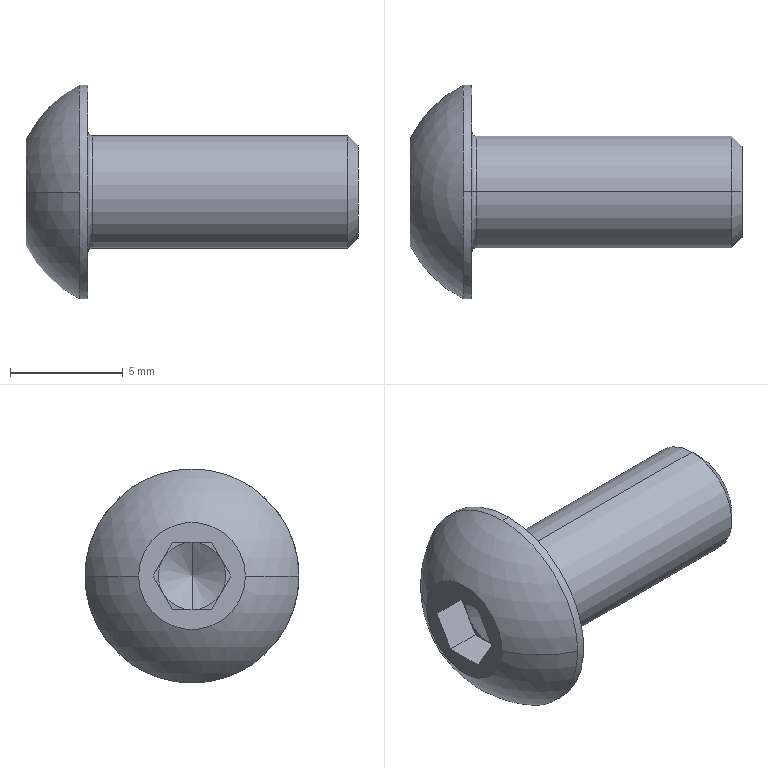Part | STEP file | SOCKET_BUTTON_HEAD_SCREW_ISO_IS | 1 solid | 27 faces | box 14.75 x 9.5 x 9.5 mm | volume 358.994 mm3 | plane 15 | cone 4 | cylinder 4 | torus 2 | sphere 2 | commonest cylinder face diameters 5 x2 9.5 x2
STEP:
#1=CARTESIAN_POINT('',(2.75,0.,2.7));
#2=VERTEX_POINT('',#1);
#3=CARTESIAN_POINT('',(2.75,0.,-2.7));
#4=VERTEX_POINT('',#3);
#5=CARTESIAN_POINT('',(2.75,0.,0.));
#6=DIRECTION('',(-1.,0.,0.));
#7=DIRECTION('',(0.,0.,1.));
#8=AXIS2_PLACEMENT_3D('',#5,#6,#7);
#9=CIRCLE('',#8,2.7);
#10=EDGE_CURVE('',#2,#4,#9,.T.);
#11=ORIENTED_EDGE('',*,*,#10,.F.);
#12=CARTESIAN_POINT('',(2.95,0.,2.5));
#13=VERTEX_POINT('',#12);
#14=CARTESIAN_POINT('',(2.95,0.,2.7));
#15=DIRECTION('',(0.,1.,0.));
#16=DIRECTION('',(0.,0.,-1.));
#17=AXIS2_PLACEMENT_3D('',#14,#15,#16);
#18=CIRCLE('',#17,0.2);
#19=EDGE_CURVE('',#13,#2,#18,.T.);
#20=ORIENTED_EDGE('',*,*,#19,.F.);
#21=CARTESIAN_POINT('',(2.95,0.,-2.5));
#22=VERTEX_POINT('',#21);
#23=CARTESIAN_POINT('',(2.95,0.,0.));
#24=DIRECTION('',(-1.,0.,0.));
#25=DIRECTION('',(0.,0.,1.));
#26=AXIS2_PLACEMENT_3D('',#23,#24,#25);
#27=CIRCLE('',#26,2.5);
#28=EDGE_CURVE('',#13,#22,#27,.T.);
#29=ORIENTED_EDGE('',*,*,#28,.T.);
#30=CARTESIAN_POINT('',(2.95,0.,-2.7));
#31=DIRECTION('',(0.,-1.,0.));
#32=DIRECTION('',(0.,0.,1.));
#33=AXIS2_PLACEMENT_3D('',#30,#31,#32);
#34=CIRCLE('',#33,0.2);
#35=EDGE_CURVE('',#22,#4,#34,.T.);
#36=ORIENTED_EDGE('',*,*,#35,.T.);
#37=EDGE_LOOP('',(#11,#20,#29,#36));
#38=FACE_OUTER_BOUND('',#37,.T.);
#39=CARTESIAN_POINT('',(2.95,0.,0.));
#40=DIRECTION('',(-1.,0.,0.));
#41=DIRECTION('',(0.,0.,1.));
#42=AXIS2_PLACEMENT_3D('',#39,#40,#41);
#43=TOROIDAL_SURFACE('',#42,2.7,0.2);
#44=ADVANCED_FACE('',(#38),#43,.F.);
#45=CARTESIAN_POINT('',(1.56,1.299,0.75));
#46=VERTEX_POINT('',#45);
#47=CARTESIAN_POINT('',(1.56,1.732,0.));
#48=VERTEX_POINT('',#47);
#49=CARTESIAN_POINT('',(1.56,1.299,0.75));
#50=DIRECTION('',(0.,0.5,-0.866));
#51=VECTOR('',#50,1000.);
#52=LINE('',#49,#51);
#53=EDGE_CURVE('',#46,#48,#52,.T.);
#54=ORIENTED_EDGE('',*,*,#53,.T.);
#55=CARTESIAN_POINT('',(1.56,1.299,-0.75));
#56=VERTEX_POINT('',#55);
#57=CARTESIAN_POINT('',(1.56,1.732,0.));
#58=DIRECTION('',(0.,-0.5,-0.866));
#59=VECTOR('',#58,1000.);
#60=LINE('',#57,#59);
#61=EDGE_CURVE('',#48,#56,#60,.T.);
#62=ORIENTED_EDGE('',*,*,#61,.T.);
#63=CARTESIAN_POINT('',(1.56,0.,0.));
#64=DIRECTION('',(1.,0.,0.));
#65=DIRECTION('',(0.,0.866,-0.5));
#66=AXIS2_PLACEMENT_3D('',#63,#64,#65);
#67=CIRCLE('',#66,1.5);
#68=EDGE_CURVE('',#56,#46,#67,.T.);
#69=ORIENTED_EDGE('',*,*,#68,.T.);
#70=EDGE_LOOP('',(#54,#62,#69));
#71=FACE_OUTER_BOUND('',#70,.T.);
#72=CARTESIAN_POINT('',(1.56,-1.732,0.));
#73=DIRECTION('',(1.,0.,0.));
#74=DIRECTION('',(0.,1.,0.));
#75=AXIS2_PLACEMENT_3D('',#72,#73,#74);
#76=PLANE('',#75);
#77=ADVANCED_FACE('',(#71),#76,.F.);
#78=CARTESIAN_POINT('',(1.56,0.866,1.5));
#79=VERTEX_POINT('',#78);
#80=CARTESIAN_POINT('',(1.56,0.866,1.5));
#81=DIRECTION('',(0.,0.5,-0.866));
#82=VECTOR('',#81,1000.);
#83=LINE('',#80,#82);
#84=EDGE_CURVE('',#79,#46,#83,.T.);
#85=ORIENTED_EDGE('',*,*,#84,.F.);
#86=CARTESIAN_POINT('',(0.,0.866,1.5));
#87=VERTEX_POINT('',#86);
#88=CARTESIAN_POINT('',(0.,0.866,1.5));
#89=DIRECTION('',(1.,0.,0.));
#90=VECTOR('',#89,1000.);
#91=LINE('',#88,#90);
#92=EDGE_CURVE('',#87,#79,#91,.T.);
#93=ORIENTED_EDGE('',*,*,#92,.F.);
#94=CARTESIAN_POINT('',(0.,1.732,0.));
#95=VERTEX_POINT('',#94);
#96=CARTESIAN_POINT('',(0.,1.732,0.));
#97=DIRECTION('',(0.,-0.5,0.866));
#98=VECTOR('',#97,1000.);
#99=LINE('',#96,#98);
#100=EDGE_CURVE('',#95,#87,#99,.T.);
#101=ORIENTED_EDGE('',*,*,#100,.F.);
#102=CARTESIAN_POINT('',(0.,1.732,0.));
#103=DIRECTION('',(1.,0.,0.));
#104=VECTOR('',#103,1000.);
#105=LINE('',#102,#104);
#106=EDGE_CURVE('',#95,#48,#105,.T.);
#107=ORIENTED_EDGE('',*,*,#106,.T.);
#108=ORIENTED_EDGE('',*,*,#53,.F.);
#109=EDGE_LOOP('',(#85,#93,#101,#107,#108));
#110=FACE_OUTER_BOUND('',#109,.T.);
#111=CARTESIAN_POINT('',(1.56,0.866,1.5));
#112=DIRECTION('',(0.,-0.866,-0.5));
#113=DIRECTION('',(0.,0.5,-0.866));
#114=AXIS2_PLACEMENT_3D('',#111,#112,#113);
#115=PLANE('',#114);
#116=ADVANCED_FACE('',(#110),#115,.T.);
#117=CARTESIAN_POINT('',(1.56,0.866,-1.5));
#118=VERTEX_POINT('',#117);
#119=CARTESIAN_POINT('',(1.56,1.299,-0.75));
#120=DIRECTION('',(0.,-0.5,-0.866));
#121=VECTOR('',#120,1000.);
#122=LINE('',#119,#121);
#123=EDGE_CURVE('',#56,#118,#122,.T.);
#124=ORIENTED_EDGE('',*,*,#123,.T.);
#125=CARTESIAN_POINT('',(1.56,0.,-1.5));
#126=VERTEX_POINT('',#125);
#127=CARTESIAN_POINT('',(1.56,0.866,-1.5));
#128=DIRECTION('',(0.,-1.,0.));
#129=VECTOR('',#128,1000.);
#130=LINE('',#127,#129);
#131=EDGE_CURVE('',#118,#126,#130,.T.);
#132=ORIENTED_EDGE('',*,*,#131,.T.);
#133=CARTESIAN_POINT('',(1.56,0.,0.));
#134=DIRECTION('',(1.,0.,0.));
#135=DIRECTION('',(0.,0.,-1.));
#136=AXIS2_PLACEMENT_3D('',#133,#134,#135);
#137=CIRCLE('',#136,1.5);
#138=EDGE_CURVE('',#126,#56,#137,.T.);
#139=ORIENTED_EDGE('',*,*,#138,.T.);
#140=EDGE_LOOP('',(#124,#132,#139));
#141=FACE_OUTER_BOUND('',#140,.T.);
#142=CARTESIAN_POINT('',(1.56,-1.732,0.));
#143=DIRECTION('',(1.,0.,0.));
#144=DIRECTION('',(0.,1.,0.));
#145=AXIS2_PLACEMENT_3D('',#142,#143,#144);
#146=PLANE('',#145);
#147=ADVANCED_FACE('',(#141),#146,.F.);
#148=ORIENTED_EDGE('',*,*,#61,.F.);
#149=ORIENTED_EDGE('',*,*,#106,.F.);
#150=CARTESIAN_POINT('',(0.,0.866,-1.5));
#151=VERTEX_POINT('',#150);
#152=CARTESIAN_POINT('',(0.,0.866,-1.5));
#153=DIRECTION('',(0.,0.5,0.866));
#154=VECTOR('',#153,1000.);
#155=LINE('',#152,#154);
#156=EDGE_CURVE('',#151,#95,#155,.T.);
#157=ORIENTED_EDGE('',*,*,#156,.F.);
#158=CARTESIAN_POINT('',(0.,0.866,-1.5));
#159=DIRECTION('',(1.,0.,0.));
#160=VECTOR('',#159,1000.);
#161=LINE('',#158,#160);
#162=EDGE_CURVE('',#151,#118,#161,.T.);
#163=ORIENTED_EDGE('',*,*,#162,.T.);
#164=ORIENTED_EDGE('',*,*,#123,.F.);
#165=EDGE_LOOP('',(#148,#149,#157,#163,#164));
#166=FACE_OUTER_BOUND('',#165,.T.);
#167=CARTESIAN_POINT('',(1.56,1.732,0.));
#168=DIRECTION('',(0.,-0.866,0.5));
#169=DIRECTION('',(-1.,0.,0.));
#170=AXIS2_PLACEMENT_3D('',#167,#168,#169);
#171=PLANE('',#170);
#172=ADVANCED_FACE('',(#166),#171,.T.);
#173=CARTESIAN_POINT('',(1.56,-0.866,-1.5));
#174=VERTEX_POINT('',#173);
#175=CARTESIAN_POINT('',(1.56,0.,-1.5));
#176=DIRECTION('',(0.,-1.,0.));
#177=VECTOR('',#176,1000.);
#178=LINE('',#175,#177);
#179=EDGE_CURVE('',#126,#174,#178,.T.);
#180=ORIENTED_EDGE('',*,*,#179,.T.);
#181=CARTESIAN_POINT('',(1.56,-1.299,-0.75));
#182=VERTEX_POINT('',#181);
#183=CARTESIAN_POINT('',(1.56,-0.866,-1.5));
#184=DIRECTION('',(0.,-0.5,0.866));
#185=VECTOR('',#184,1000.);
#186=LINE('',#183,#185);
#187=EDGE_CURVE('',#174,#182,#186,.T.);
#188=ORIENTED_EDGE('',*,*,#187,.T.);
#189=CARTESIAN_POINT('',(1.56,0.,0.));
#190=DIRECTION('',(1.,0.,0.));
#191=DIRECTION('',(0.,-0.866,-0.5));
#192=AXIS2_PLACEMENT_3D('',#189,#190,#191);
#193=CIRCLE('',#192,1.5);
#194=EDGE_CURVE('',#182,#126,#193,.T.);
#195=ORIENTED_EDGE('',*,*,#194,.T.);
#196=EDGE_LOOP('',(#180,#188,#195));
#197=FACE_OUTER_BOUND('',#196,.T.);
#198=CARTESIAN_POINT('',(1.56,-1.732,0.));
#199=DIRECTION('',(1.,0.,0.));
#200=DIRECTION('',(0.,1.,0.));
#201=AXIS2_PLACEMENT_3D('',#198,#199,#200);
#202=PLANE('',#201);
#203=ADVANCED_FACE('',(#197),#202,.F.);
#204=ORIENTED_EDGE('',*,*,#131,.F.);
#205=ORIENTED_EDGE('',*,*,#162,.F.);
#206=CARTESIAN_POINT('',(0.,-0.866,-1.5));
#207=VERTEX_POINT('',#206);
#208=CARTESIAN_POINT('',(0.,0.866,-1.5));
#209=DIRECTION('',(0.,-1.,0.));
#210=VECTOR('',#209,1000.);
#211=LINE('',#208,#210);
#212=EDGE_CURVE('',#151,#207,#211,.T.);
#213=ORIENTED_EDGE('',*,*,#212,.T.);
#214=CARTESIAN_POINT('',(0.,-0.866,-1.5));
#215=DIRECTION('',(1.,0.,0.));
#216=VECTOR('',#215,1000.);
#217=LINE('',#214,#216);
#218=EDGE_CURVE('',#207,#174,#217,.T.);
#219=ORIENTED_EDGE('',*,*,#218,.T.);
#220=ORIENTED_EDGE('',*,*,#179,.F.);
#221=EDGE_LOOP('',(#204,#205,#213,#219,#220));
#222=FACE_OUTER_BOUND('',#221,.T.);
#223=CARTESIAN_POINT('',(1.56,0.866,-1.5));
#224=DIRECTION('',(0.,0.,1.));
#225=DIRECTION('',(1.,0.,0.));
#226=AXIS2_PLACEMENT_3D('',#223,#224,#225);
#227=PLANE('',#226);
#228=ADVANCED_FACE('',(#222),#227,.T.);
#229=CARTESIAN_POINT('',(1.56,-1.732,0.));
#230=VERTEX_POINT('',#229);
#231=CARTESIAN_POINT('',(1.56,-1.299,-0.75));
#232=DIRECTION('',(0.,-0.5,0.866));
#233=VECTOR('',#232,1000.);
#234=LINE('',#231,#233);
#235=EDGE_CURVE('',#182,#230,#234,.T.);
#236=ORIENTED_EDGE('',*,*,#235,.T.);
#237=CARTESIAN_POINT('',(1.56,-1.299,0.75));
#238=VERTEX_POINT('',#237);
#239=CARTESIAN_POINT('',(1.56,-1.732,0.));
#240=DIRECTION('',(0.,0.5,0.866));
#241=VECTOR('',#240,1000.);
#242=LINE('',#239,#241);
#243=EDGE_CURVE('',#230,#238,#242,.T.);
#244=ORIENTED_EDGE('',*,*,#243,.T.);
#245=CARTESIAN_POINT('',(1.56,0.,0.));
#246=DIRECTION('',(1.,0.,0.));
#247=DIRECTION('',(0.,-0.866,0.5));
#248=AXIS2_PLACEMENT_3D('',#245,#246,#247);
#249=CIRCLE('',#248,1.5);
#250=EDGE_CURVE('',#238,#182,#249,.T.);
#251=ORIENTED_EDGE('',*,*,#250,.T.);
#252=EDGE_LOOP('',(#236,#244,#251));
#253=FACE_OUTER_BOUND('',#252,.T.);
#254=CARTESIAN_POINT('',(1.56,-1.732,0.));
#255=DIRECTION('',(1.,0.,0.));
#256=DIRECTION('',(0.,1.,0.));
#257=AXIS2_PLACEMENT_3D('',#254,#255,#256);
#258=PLANE('',#257);
#259=ADVANCED_FACE('',(#253),#258,.F.);
#260=ORIENTED_EDGE('',*,*,#187,.F.);
#261=ORIENTED_EDGE('',*,*,#218,.F.);
#262=CARTESIAN_POINT('',(0.,-1.732,0.));
#263=VERTEX_POINT('',#262);
#264=CARTESIAN_POINT('',(0.,-1.732,0.));
#265=DIRECTION('',(0.,0.5,-0.866));
#266=VECTOR('',#265,1000.);
#267=LINE('',#264,#266);
#268=EDGE_CURVE('',#263,#207,#267,.T.);
#269=ORIENTED_EDGE('',*,*,#268,.F.);
#270=CARTESIAN_POINT('',(0.,-1.732,0.));
#271=DIRECTION('',(1.,0.,0.));
#272=VECTOR('',#271,1000.);
#273=LINE('',#270,#272);
#274=EDGE_CURVE('',#263,#230,#273,.T.);
#275=ORIENTED_EDGE('',*,*,#274,.T.);
#276=ORIENTED_EDGE('',*,*,#235,.F.);
#277=EDGE_LOOP('',(#260,#261,#269,#275,#276));
#278=FACE_OUTER_BOUND('',#277,.T.);
#279=CARTESIAN_POINT('',(1.56,-0.866,-1.5));
#280=DIRECTION('',(0.,0.866,0.5));
#281=DIRECTION('',(1.,0.,0.));
#282=AXIS2_PLACEMENT_3D('',#279,#280,#281);
#283=PLANE('',#282);
#284=ADVANCED_FACE('',(#278),#283,.T.);
#285=ORIENTED_EDGE('',*,*,#243,.F.);
#286=ORIENTED_EDGE('',*,*,#274,.F.);
#287=CARTESIAN_POINT('',(0.,-0.866,1.5));
#288=VERTEX_POINT('',#287);
#289=CARTESIAN_POINT('',(0.,-0.866,1.5));
#290=DIRECTION('',(0.,-0.5,-0.866));
#291=VECTOR('',#290,1000.);
#292=LINE('',#289,#291);
#293=EDGE_CURVE('',#288,#263,#292,.T.);
#294=ORIENTED_EDGE('',*,*,#293,.F.);
#295=CARTESIAN_POINT('',(1.56,-0.866,1.5));
#296=VERTEX_POINT('',#295);
#297=CARTESIAN_POINT('',(0.,-0.866,1.5));
#298=DIRECTION('',(1.,0.,0.));
#299=VECTOR('',#298,1000.);
#300=LINE('',#297,#299);
#301=EDGE_CURVE('',#288,#296,#300,.T.);
#302=ORIENTED_EDGE('',*,*,#301,.T.);
#303=CARTESIAN_POINT('',(1.56,-1.299,0.75));
#304=DIRECTION('',(0.,0.5,0.866));
#305=VECTOR('',#304,1000.);
#306=LINE('',#303,#305);
#307=EDGE_CURVE('',#238,#296,#306,.T.);
#308=ORIENTED_EDGE('',*,*,#307,.F.);
#309=EDGE_LOOP('',(#285,#286,#294,#302,#308));
#310=FACE_OUTER_BOUND('',#309,.T.);
#311=CARTESIAN_POINT('',(1.56,-1.732,0.));
#312=DIRECTION('',(0.,0.866,-0.5));
#313=DIRECTION('',(-1.,0.,0.));
#314=AXIS2_PLACEMENT_3D('',#311,#312,#313);
#315=PLANE('',#314);
#316=ADVANCED_FACE('',(#310),#315,.T.);
#317=ORIENTED_EDGE('',*,*,#307,.T.);
#318=CARTESIAN_POINT('',(1.56,0.,1.5));
#319=VERTEX_POINT('',#318);
#320=CARTESIAN_POINT('',(1.56,-0.866,1.5));
#321=DIRECTION('',(0.,1.,0.));
#322=VECTOR('',#321,1000.);
#323=LINE('',#320,#322);
#324=EDGE_CURVE('',#296,#319,#323,.T.);
#325=ORIENTED_EDGE('',*,*,#324,.T.);
#326=CARTESIAN_POINT('',(1.56,0.,0.));
#327=DIRECTION('',(1.,0.,0.));
#328=DIRECTION('',(0.,0.,1.));
#329=AXIS2_PLACEMENT_3D('',#326,#327,#328);
#330=CIRCLE('',#329,1.5);
#331=EDGE_CURVE('',#319,#238,#330,.T.);
#332=ORIENTED_EDGE('',*,*,#331,.T.);
#333=EDGE_LOOP('',(#317,#325,#332));
#334=FACE_OUTER_BOUND('',#333,.T.);
#335=CARTESIAN_POINT('',(1.56,-1.732,0.));
#336=DIRECTION('',(1.,0.,0.));
#337=DIRECTION('',(0.,1.,0.));
#338=AXIS2_PLACEMENT_3D('',#335,#336,#337);
#339=PLANE('',#338);
#340=ADVANCED_FACE('',(#334),#339,.F.);
#341=CARTESIAN_POINT('',(2.426,0.,0.));
#342=VERTEX_POINT('',#341);
#343=CARTESIAN_POINT('',(1.56,0.,-1.5));
#344=DIRECTION('',(0.5,0.,0.866));
#345=VECTOR('',#344,1000.);
#346=LINE('',#343,#345);
#347=EDGE_CURVE('',#126,#342,#346,.T.);
#348=ORIENTED_EDGE('',*,*,#347,.F.);
#349=ORIENTED_EDGE('',*,*,#194,.F.);
#350=ORIENTED_EDGE('',*,*,#250,.F.);
#351=ORIENTED_EDGE('',*,*,#331,.F.);
#352=CARTESIAN_POINT('',(1.56,0.,1.5));
#353=DIRECTION('',(0.5,0.,-0.866));
#354=VECTOR('',#353,1000.);
#355=LINE('',#352,#354);
#356=EDGE_CURVE('',#319,#342,#355,.T.);
#357=ORIENTED_EDGE('',*,*,#356,.T.);
#358=EDGE_LOOP('',(#348,#349,#350,#351,#357));
#359=FACE_OUTER_BOUND('',#358,.T.);
#360=CARTESIAN_POINT('',(1.984,0.,0.));
#361=DIRECTION('',(-1.,0.,0.));
#362=DIRECTION('',(0.,0.,1.));
#363=AXIS2_PLACEMENT_3D('',#360,#361,#362);
#364=CONICAL_SURFACE('',#363,0.765,1.047);
#365=ADVANCED_FACE('',(#359),#364,.F.);
#366=ORIENTED_EDGE('',*,*,#356,.F.);
#367=CARTESIAN_POINT('',(1.56,0.,0.));
#368=DIRECTION('',(1.,0.,0.));
#369=DIRECTION('',(0.,0.866,0.5));
#370=AXIS2_PLACEMENT_3D('',#367,#368,#369);
#371=CIRCLE('',#370,1.5);
#372=EDGE_CURVE('',#46,#319,#371,.T.);
#373=ORIENTED_EDGE('',*,*,#372,.F.);
#374=ORIENTED_EDGE('',*,*,#68,.F.);
#375=ORIENTED_EDGE('',*,*,#138,.F.);
#376=ORIENTED_EDGE('',*,*,#347,.T.);
#377=EDGE_LOOP('',(#366,#373,#374,#375,#376));
#378=FACE_OUTER_BOUND('',#377,.T.);
#379=CARTESIAN_POINT('',(1.984,0.,0.));
#380=DIRECTION('',(-1.,0.,0.));
#381=DIRECTION('',(0.,0.,1.));
#382=AXIS2_PLACEMENT_3D('',#379,#380,#381);
#383=CONICAL_SURFACE('',#382,0.765,1.047);
#384=ADVANCED_FACE('',(#378),#383,.F.);
#385=CARTESIAN_POINT('',(1.56,0.,1.5));
#386=DIRECTION('',(0.,1.,0.));
#387=VECTOR('',#386,1000.);
#388=LINE('',#385,#387);
#389=EDGE_CURVE('',#319,#79,#388,.T.);
#390=ORIENTED_EDGE('',*,*,#389,.T.);
#391=ORIENTED_EDGE('',*,*,#84,.T.);
#392=ORIENTED_EDGE('',*,*,#372,.T.);
#393=EDGE_LOOP('',(#390,#391,#392));
#394=FACE_OUTER_BOUND('',#393,.T.);
#395=CARTESIAN_POINT('',(1.56,-1.732,0.));
#396=DIRECTION('',(1.,0.,0.));
#397=DIRECTION('',(0.,1.,0.));
#398=AXIS2_PLACEMENT_3D('',#395,#396,#397);
#399=PLANE('',#398);
#400=ADVANCED_FACE('',(#394),#399,.F.);
#401=ORIENTED_EDGE('',*,*,#324,.F.);
#402=ORIENTED_EDGE('',*,*,#301,.F.);
#403=CARTESIAN_POINT('',(0.,-0.866,1.5));
#404=DIRECTION('',(0.,1.,0.));
#405=VECTOR('',#404,1000.);
#406=LINE('',#403,#405);
#407=EDGE_CURVE('',#288,#87,#406,.T.);
#408=ORIENTED_EDGE('',*,*,#407,.T.);
#409=ORIENTED_EDGE('',*,*,#92,.T.);
#410=ORIENTED_EDGE('',*,*,#389,.F.);
#411=EDGE_LOOP('',(#401,#402,#408,#409,#410));
#412=FACE_OUTER_BOUND('',#411,.T.);
#413=CARTESIAN_POINT('',(1.56,-0.866,1.5));
#414=DIRECTION('',(0.,0.,-1.));
#415=DIRECTION('',(0.,-1.,0.));
#416=AXIS2_PLACEMENT_3D('',#413,#414,#415);
#417=PLANE('',#416);
#418=ADVANCED_FACE('',(#412),#417,.T.);
#419=ORIENTED_EDGE('',*,*,#293,.T.);
#420=ORIENTED_EDGE('',*,*,#268,.T.);
#421=ORIENTED_EDGE('',*,*,#212,.F.);
#422=ORIENTED_EDGE('',*,*,#156,.T.);
#423=ORIENTED_EDGE('',*,*,#100,.T.);
#424=ORIENTED_EDGE('',*,*,#407,.F.);
#425=EDGE_LOOP('',(#419,#420,#421,#422,#423,#424));
#426=FACE_BOUND('',#425,.T.);
#427=CARTESIAN_POINT('',(0.,-2.375,0.));
#428=VERTEX_POINT('',#427);
#429=CARTESIAN_POINT('',(0.,2.375,0.));
#430=VERTEX_POINT('',#429);
#431=CARTESIAN_POINT('',(0.,0.,0.));
#432=DIRECTION('',(1.,0.,0.));
#433=DIRECTION('',(0.,-1.,0.));
#434=AXIS2_PLACEMENT_3D('',#431,#432,#433);
#435=CIRCLE('',#434,2.375);
#436=EDGE_CURVE('',#428,#430,#435,.T.);
#437=ORIENTED_EDGE('',*,*,#436,.F.);
#438=CARTESIAN_POINT('',(0.,0.,0.));
#439=DIRECTION('',(-1.,0.,0.));
#440=DIRECTION('',(0.,-1.,0.));
#441=AXIS2_PLACEMENT_3D('',#438,#439,#440);
#442=CIRCLE('',#441,2.375);
#443=EDGE_CURVE('',#428,#430,#442,.T.);
#444=ORIENTED_EDGE('',*,*,#443,.T.);
#445=EDGE_LOOP('',(#437,#444));
#446=FACE_OUTER_BOUND('',#445,.T.);
#447=CARTESIAN_POINT('',(0.,0.,0.));
#448=DIRECTION('',(-1.,0.,0.));
#449=DIRECTION('',(0.,0.,1.));
#450=AXIS2_PLACEMENT_3D('',#447,#448,#449);
#451=PLANE('',#450);
#452=ADVANCED_FACE('',(#426,#446),#451,.T.);
#453=CARTESIAN_POINT('',(2.37,-4.75,0.));
#454=VERTEX_POINT('',#453);
#455=CARTESIAN_POINT('',(2.37,0.,4.75));
#456=VERTEX_POINT('',#455);
#457=CARTESIAN_POINT('',(2.37,0.,0.));
#458=DIRECTION('',(-1.,0.,0.));
#459=DIRECTION('',(0.,-1.,0.));
#460=AXIS2_PLACEMENT_3D('',#457,#458,#459);
#461=CIRCLE('',#460,4.75);
#462=EDGE_CURVE('',#454,#456,#461,.T.);
#463=ORIENTED_EDGE('',*,*,#462,.T.);
#464=CARTESIAN_POINT('',(2.37,4.75,0.));
#465=VERTEX_POINT('',#464);
#466=CARTESIAN_POINT('',(2.37,0.,0.));
#467=DIRECTION('',(-1.,0.,0.));
#468=DIRECTION('',(0.,0.,1.));
#469=AXIS2_PLACEMENT_3D('',#466,#467,#468);
#470=CIRCLE('',#469,4.75);
#471=EDGE_CURVE('',#456,#465,#470,.T.);
#472=ORIENTED_EDGE('',*,*,#471,.T.);
#473=CARTESIAN_POINT('',(4.755,0.,0.));
#474=DIRECTION('',(0.,0.,-1.));
#475=DIRECTION('',(-0.8946,0.4468,0.));
#476=AXIS2_PLACEMENT_3D('',#473,#474,#475);
#477=CIRCLE('',#476,5.315);
#478=EDGE_CURVE('',#430,#465,#477,.T.);
#479=ORIENTED_EDGE('',*,*,#478,.F.);
#480=ORIENTED_EDGE('',*,*,#443,.F.);
#481=CARTESIAN_POINT('',(4.755,0.,0.));
#482=DIRECTION('',(0.,0.,1.));
#483=DIRECTION('',(-0.8946,-0.4468,0.));
#484=AXIS2_PLACEMENT_3D('',#481,#482,#483);
#485=CIRCLE('',#484,5.315);
#486=EDGE_CURVE('',#428,#454,#485,.T.);
#487=ORIENTED_EDGE('',*,*,#486,.T.);
#488=EDGE_LOOP('',(#463,#472,#479,#480,#487));
#489=FACE_OUTER_BOUND('',#488,.T.);
#490=CARTESIAN_POINT('',(4.755,0.,0.));
#491=DIRECTION('',(0.,0.,1.));
#492=DIRECTION('',(0.,1.,0.));
#493=AXIS2_PLACEMENT_3D('',#490,#491,#492);
#494=SPHERICAL_SURFACE('',#493,5.315);
#495=ADVANCED_FACE('',(#489),#494,.T.);
#496=CARTESIAN_POINT('',(2.37,0.,-4.75));
#497=VERTEX_POINT('',#496);
#498=CARTESIAN_POINT('',(2.37,0.,0.));
#499=DIRECTION('',(-1.,0.,0.));
#500=DIRECTION('',(0.,0.,-1.));
#501=AXIS2_PLACEMENT_3D('',#498,#499,#500);
#502=CIRCLE('',#501,4.75);
#503=EDGE_CURVE('',#497,#454,#502,.T.);
#504=ORIENTED_EDGE('',*,*,#503,.T.);
#505=ORIENTED_EDGE('',*,*,#486,.F.);
#506=ORIENTED_EDGE('',*,*,#436,.T.);
#507=ORIENTED_EDGE('',*,*,#478,.T.);
#508=CARTESIAN_POINT('',(2.37,0.,0.));
#509=DIRECTION('',(-1.,0.,0.));
#510=DIRECTION('',(0.,1.,0.));
#511=AXIS2_PLACEMENT_3D('',#508,#509,#510);
#512=CIRCLE('',#511,4.75);
#513=EDGE_CURVE('',#465,#497,#512,.T.);
#514=ORIENTED_EDGE('',*,*,#513,.T.);
#515=EDGE_LOOP('',(#504,#505,#506,#507,#514));
#516=FACE_OUTER_BOUND('',#515,.T.);
#517=CARTESIAN_POINT('',(4.755,0.,0.));
#518=DIRECTION('',(0.,0.,1.));
#519=DIRECTION('',(-0.4468,-0.8946,0.));
#520=AXIS2_PLACEMENT_3D('',#517,#518,#519);
#521=SPHERICAL_SURFACE('',#520,5.315);
#522=ADVANCED_FACE('',(#516),#521,.T.);
#523=CARTESIAN_POINT('',(2.75,0.,4.75));
#524=VERTEX_POINT('',#523);
#525=CARTESIAN_POINT('',(2.75,0.,-4.75));
#526=VERTEX_POINT('',#525);
#527=CARTESIAN_POINT('',(2.75,0.,0.));
#528=DIRECTION('',(1.,0.,0.));
#529=DIRECTION('',(0.,0.,1.));
#530=AXIS2_PLACEMENT_3D('',#527,#528,#529);
#531=CIRCLE('',#530,4.75);
#532=EDGE_CURVE('',#524,#526,#531,.T.);
#533=ORIENTED_EDGE('',*,*,#532,.F.);
#534=CARTESIAN_POINT('',(2.37,0.,4.75));
#535=DIRECTION('',(1.,0.,0.));
#536=VECTOR('',#535,1000.);
#537=LINE('',#534,#536);
#538=EDGE_CURVE('',#456,#524,#537,.T.);
#539=ORIENTED_EDGE('',*,*,#538,.F.);
#540=ORIENTED_EDGE('',*,*,#462,.F.);
#541=ORIENTED_EDGE('',*,*,#503,.F.);
#542=CARTESIAN_POINT('',(2.37,0.,-4.75));
#543=DIRECTION('',(1.,0.,0.));
#544=VECTOR('',#543,1000.);
#545=LINE('',#542,#544);
#546=EDGE_CURVE('',#497,#526,#545,.T.);
#547=ORIENTED_EDGE('',*,*,#546,.T.);
#548=EDGE_LOOP('',(#533,#539,#540,#541,#547));
#549=FACE_OUTER_BOUND('',#548,.T.);
#550=CARTESIAN_POINT('',(0.,0.,0.));
#551=DIRECTION('',(-1.,0.,0.));
#552=DIRECTION('',(0.,0.,1.));
#553=AXIS2_PLACEMENT_3D('',#550,#551,#552);
#554=CYLINDRICAL_SURFACE('',#553,4.75);
#555=ADVANCED_FACE('',(#549),#554,.T.);
#556=ORIENTED_EDGE('',*,*,#546,.F.);
#557=ORIENTED_EDGE('',*,*,#513,.F.);
#558=ORIENTED_EDGE('',*,*,#471,.F.);
#559=ORIENTED_EDGE('',*,*,#538,.T.);
#560=CARTESIAN_POINT('',(2.75,0.,0.));
#561=DIRECTION('',(1.,0.,0.));
#562=DIRECTION('',(0.,0.,-1.));
#563=AXIS2_PLACEMENT_3D('',#560,#561,#562);
#564=CIRCLE('',#563,4.75);
#565=EDGE_CURVE('',#526,#524,#564,.T.);
#566=ORIENTED_EDGE('',*,*,#565,.F.);
#567=EDGE_LOOP('',(#556,#557,#558,#559,#566));
#568=FACE_OUTER_BOUND('',#567,.T.);
#569=CARTESIAN_POINT('',(0.,0.,0.));
#570=DIRECTION('',(-1.,0.,0.));
#571=DIRECTION('',(0.,0.,1.));
#572=AXIS2_PLACEMENT_3D('',#569,#570,#571);
#573=CYLINDRICAL_SURFACE('',#572,4.75);
#574=ADVANCED_FACE('',(#568),#573,.T.);
#575=CARTESIAN_POINT('',(2.75,0.,0.));
#576=DIRECTION('',(-1.,0.,0.));
#577=DIRECTION('',(0.,0.,-1.));
#578=AXIS2_PLACEMENT_3D('',#575,#576,#577);
#579=CIRCLE('',#578,2.7);
#580=EDGE_CURVE('',#4,#2,#579,.T.);
#581=ORIENTED_EDGE('',*,*,#580,.T.);
#582=ORIENTED_EDGE('',*,*,#10,.T.);
#583=EDGE_LOOP('',(#581,#582));
#584=FACE_BOUND('',#583,.T.);
#585=ORIENTED_EDGE('',*,*,#532,.T.);
#586=ORIENTED_EDGE('',*,*,#565,.T.);
#587=EDGE_LOOP('',(#585,#586));
#588=FACE_OUTER_BOUND('',#587,.T.);
#589=CARTESIAN_POINT('',(2.75,2.5,0.));
#590=DIRECTION('',(-1.,0.,0.));
#591=DIRECTION('',(0.,0.,1.));
#592=AXIS2_PLACEMENT_3D('',#589,#590,#591);
#593=PLANE('',#592);
#594=ADVANCED_FACE('',(#584,#588),#593,.F.);
#595=ORIENTED_EDGE('',*,*,#35,.F.);
#596=CARTESIAN_POINT('',(2.95,0.,0.));
#597=DIRECTION('',(-1.,0.,0.));
#598=DIRECTION('',(0.,0.,-1.));
#599=AXIS2_PLACEMENT_3D('',#596,#597,#598);
#600=CIRCLE('',#599,2.5);
#601=EDGE_CURVE('',#22,#13,#600,.T.);
#602=ORIENTED_EDGE('',*,*,#601,.T.);
#603=ORIENTED_EDGE('',*,*,#19,.T.);
#604=ORIENTED_EDGE('',*,*,#580,.F.);
#605=EDGE_LOOP('',(#595,#602,#603,#604));
#606=FACE_OUTER_BOUND('',#605,.T.);
#607=CARTESIAN_POINT('',(2.95,0.,0.));
#608=DIRECTION('',(-1.,0.,0.));
#609=DIRECTION('',(0.,0.,1.));
#610=AXIS2_PLACEMENT_3D('',#607,#608,#609);
#611=TOROIDAL_SURFACE('',#610,2.7,0.2);
#612=ADVANCED_FACE('',(#606),#611,.F.);
#613=CARTESIAN_POINT('',(14.305,0.,2.5));
#614=VERTEX_POINT('',#613);
#615=CARTESIAN_POINT('',(14.305,0.,-2.5));
#616=VERTEX_POINT('',#615);
#617=CARTESIAN_POINT('',(14.305,0.,0.));
#618=DIRECTION('',(1.,0.,0.));
#619=DIRECTION('',(0.,0.,1.));
#620=AXIS2_PLACEMENT_3D('',#617,#618,#619);
#621=CIRCLE('',#620,2.5);
#622=EDGE_CURVE('',#614,#616,#621,.T.);
#623=ORIENTED_EDGE('',*,*,#622,.F.);
#624=CARTESIAN_POINT('',(2.95,0.,2.5));
#625=DIRECTION('',(1.,0.,0.));
#626=VECTOR('',#625,1000.);
#627=LINE('',#624,#626);
#628=EDGE_CURVE('',#13,#614,#627,.T.);
#629=ORIENTED_EDGE('',*,*,#628,.F.);
#630=ORIENTED_EDGE('',*,*,#601,.F.);
#631=CARTESIAN_POINT('',(2.95,0.,-2.5));
#632=DIRECTION('',(1.,0.,0.));
#633=VECTOR('',#632,1000.);
#634=LINE('',#631,#633);
#635=EDGE_CURVE('',#22,#616,#634,.T.);
#636=ORIENTED_EDGE('',*,*,#635,.T.);
#637=EDGE_LOOP('',(#623,#629,#630,#636));
#638=FACE_OUTER_BOUND('',#637,.T.);
#639=CARTESIAN_POINT('',(0.,0.,0.));
#640=DIRECTION('',(-1.,0.,0.));
#641=DIRECTION('',(0.,0.,1.));
#642=AXIS2_PLACEMENT_3D('',#639,#640,#641);
#643=CYLINDRICAL_SURFACE('',#642,2.5);
#644=ADVANCED_FACE('',(#638),#643,.T.);
#645=CARTESIAN_POINT('',(14.75,0.,2.055));
#646=VERTEX_POINT('',#645);
#647=CARTESIAN_POINT('',(14.75,0.,-2.055));
#648=VERTEX_POINT('',#647);
#649=CARTESIAN_POINT('',(14.75,0.,0.));
#650=DIRECTION('',(1.,0.,0.));
#651=DIRECTION('',(0.,0.,1.));
#652=AXIS2_PLACEMENT_3D('',#649,#650,#651);
#653=CIRCLE('',#652,2.055);
#654=EDGE_CURVE('',#646,#648,#653,.T.);
#655=ORIENTED_EDGE('',*,*,#654,.F.);
#656=CARTESIAN_POINT('',(14.305,0.,2.5));
#657=DIRECTION('',(0.7071,0.,-0.7071));
#658=VECTOR('',#657,1000.);
#659=LINE('',#656,#658);
#660=EDGE_CURVE('',#614,#646,#659,.T.);
#661=ORIENTED_EDGE('',*,*,#660,.F.);
#662=ORIENTED_EDGE('',*,*,#622,.T.);
#663=CARTESIAN_POINT('',(14.305,0.,-2.5));
#664=DIRECTION('',(0.7071,0.,0.7071));
#665=VECTOR('',#664,1000.);
#666=LINE('',#663,#665);
#667=EDGE_CURVE('',#616,#648,#666,.T.);
#668=ORIENTED_EDGE('',*,*,#667,.T.);
#669=EDGE_LOOP('',(#655,#661,#662,#668));
#670=FACE_OUTER_BOUND('',#669,.T.);
#671=CARTESIAN_POINT('',(14.527,0.,0.));
#672=DIRECTION('',(-1.,0.,0.));
#673=DIRECTION('',(0.,0.,1.));
#674=AXIS2_PLACEMENT_3D('',#671,#672,#673);
#675=CONICAL_SURFACE('',#674,2.277,0.7854);
#676=ADVANCED_FACE('',(#670),#675,.T.);
#677=ORIENTED_EDGE('',*,*,#654,.T.);
#678=CARTESIAN_POINT('',(14.75,0.,0.));
#679=DIRECTION('',(1.,0.,0.));
#680=DIRECTION('',(0.,0.,-1.));
#681=AXIS2_PLACEMENT_3D('',#678,#679,#680);
#682=CIRCLE('',#681,2.055);
#683=EDGE_CURVE('',#648,#646,#682,.T.);
#684=ORIENTED_EDGE('',*,*,#683,.T.);
#685=EDGE_LOOP('',(#677,#684));
#686=FACE_OUTER_BOUND('',#685,.T.);
#687=CARTESIAN_POINT('',(14.75,0.,0.));
#688=DIRECTION('',(-1.,0.,0.));
#689=DIRECTION('',(0.,0.,1.));
#690=AXIS2_PLACEMENT_3D('',#687,#688,#689);
#691=PLANE('',#690);
#692=ADVANCED_FACE('',(#686),#691,.F.);
#693=ORIENTED_EDGE('',*,*,#667,.F.);
#694=CARTESIAN_POINT('',(14.305,0.,0.));
#695=DIRECTION('',(1.,0.,0.));
#696=DIRECTION('',(0.,0.,-1.));
#697=AXIS2_PLACEMENT_3D('',#694,#695,#696);
#698=CIRCLE('',#697,2.5);
#699=EDGE_CURVE('',#616,#614,#698,.T.);
#700=ORIENTED_EDGE('',*,*,#699,.T.);
#701=ORIENTED_EDGE('',*,*,#660,.T.);
#702=ORIENTED_EDGE('',*,*,#683,.F.);
#703=EDGE_LOOP('',(#693,#700,#701,#702));
#704=FACE_OUTER_BOUND('',#703,.T.);
#705=CARTESIAN_POINT('',(14.527,0.,0.));
#706=DIRECTION('',(-1.,0.,0.));
#707=DIRECTION('',(0.,0.,1.));
#708=AXIS2_PLACEMENT_3D('',#705,#706,#707);
#709=CONICAL_SURFACE('',#708,2.277,0.7854);
#710=ADVANCED_FACE('',(#704),#709,.T.);
#711=ORIENTED_EDGE('',*,*,#635,.F.);
#712=ORIENTED_EDGE('',*,*,#28,.F.);
#713=ORIENTED_EDGE('',*,*,#628,.T.);
#714=ORIENTED_EDGE('',*,*,#699,.F.);
#715=EDGE_LOOP('',(#711,#712,#713,#714));
#716=FACE_OUTER_BOUND('',#715,.T.);
#717=CARTESIAN_POINT('',(0.,0.,0.));
#718=DIRECTION('',(-1.,0.,0.));
#719=DIRECTION('',(0.,0.,1.));
#720=AXIS2_PLACEMENT_3D('',#717,#718,#719);
#721=CYLINDRICAL_SURFACE('',#720,2.5);
#722=ADVANCED_FACE('',(#716),#721,.T.);
#723=CLOSED_SHELL('',(#44,#77,#116,#147,#172,#203,#228,#259,#284,#316,#340,#365,#384,#400,#418,#452,#495,#522,#555,#574,#594,#612,#644,#676,#692,#710,#722));
#724=MANIFOLD_SOLID_BREP('',#723);
#725=CARTESIAN_POINT('',(0.,0.,0.));
#726=DIRECTION('',(0.,0.,1.));
#727=DIRECTION('',(1.,0.,0.));
#728=AXIS2_PLACEMENT_3D('',#725,#726,#727);
#729=(LENGTH_UNIT()NAMED_UNIT(*)SI_UNIT(.MILLI.,.METRE.));
#730=UNCERTAINTY_MEASURE_WITH_UNIT(LENGTH_MEASURE(0.00001),#729,'','');
#731=(NAMED_UNIT(*)PLANE_ANGLE_UNIT()SI_UNIT($,.RADIAN.));
#732=(NAMED_UNIT(*)SI_UNIT($,.STERADIAN.)SOLID_ANGLE_UNIT());
#733=(GEOMETRIC_REPRESENTATION_CONTEXT(3)GLOBAL_UNCERTAINTY_ASSIGNED_CONTEXT((#730))GLOBAL_UNIT_ASSIGNED_CONTEXT((#729,#731,#732))REPRESENTATION_CONTEXT('',''));
#734=ADVANCED_BREP_SHAPE_REPRESENTATION('',(#724,#728),#733);